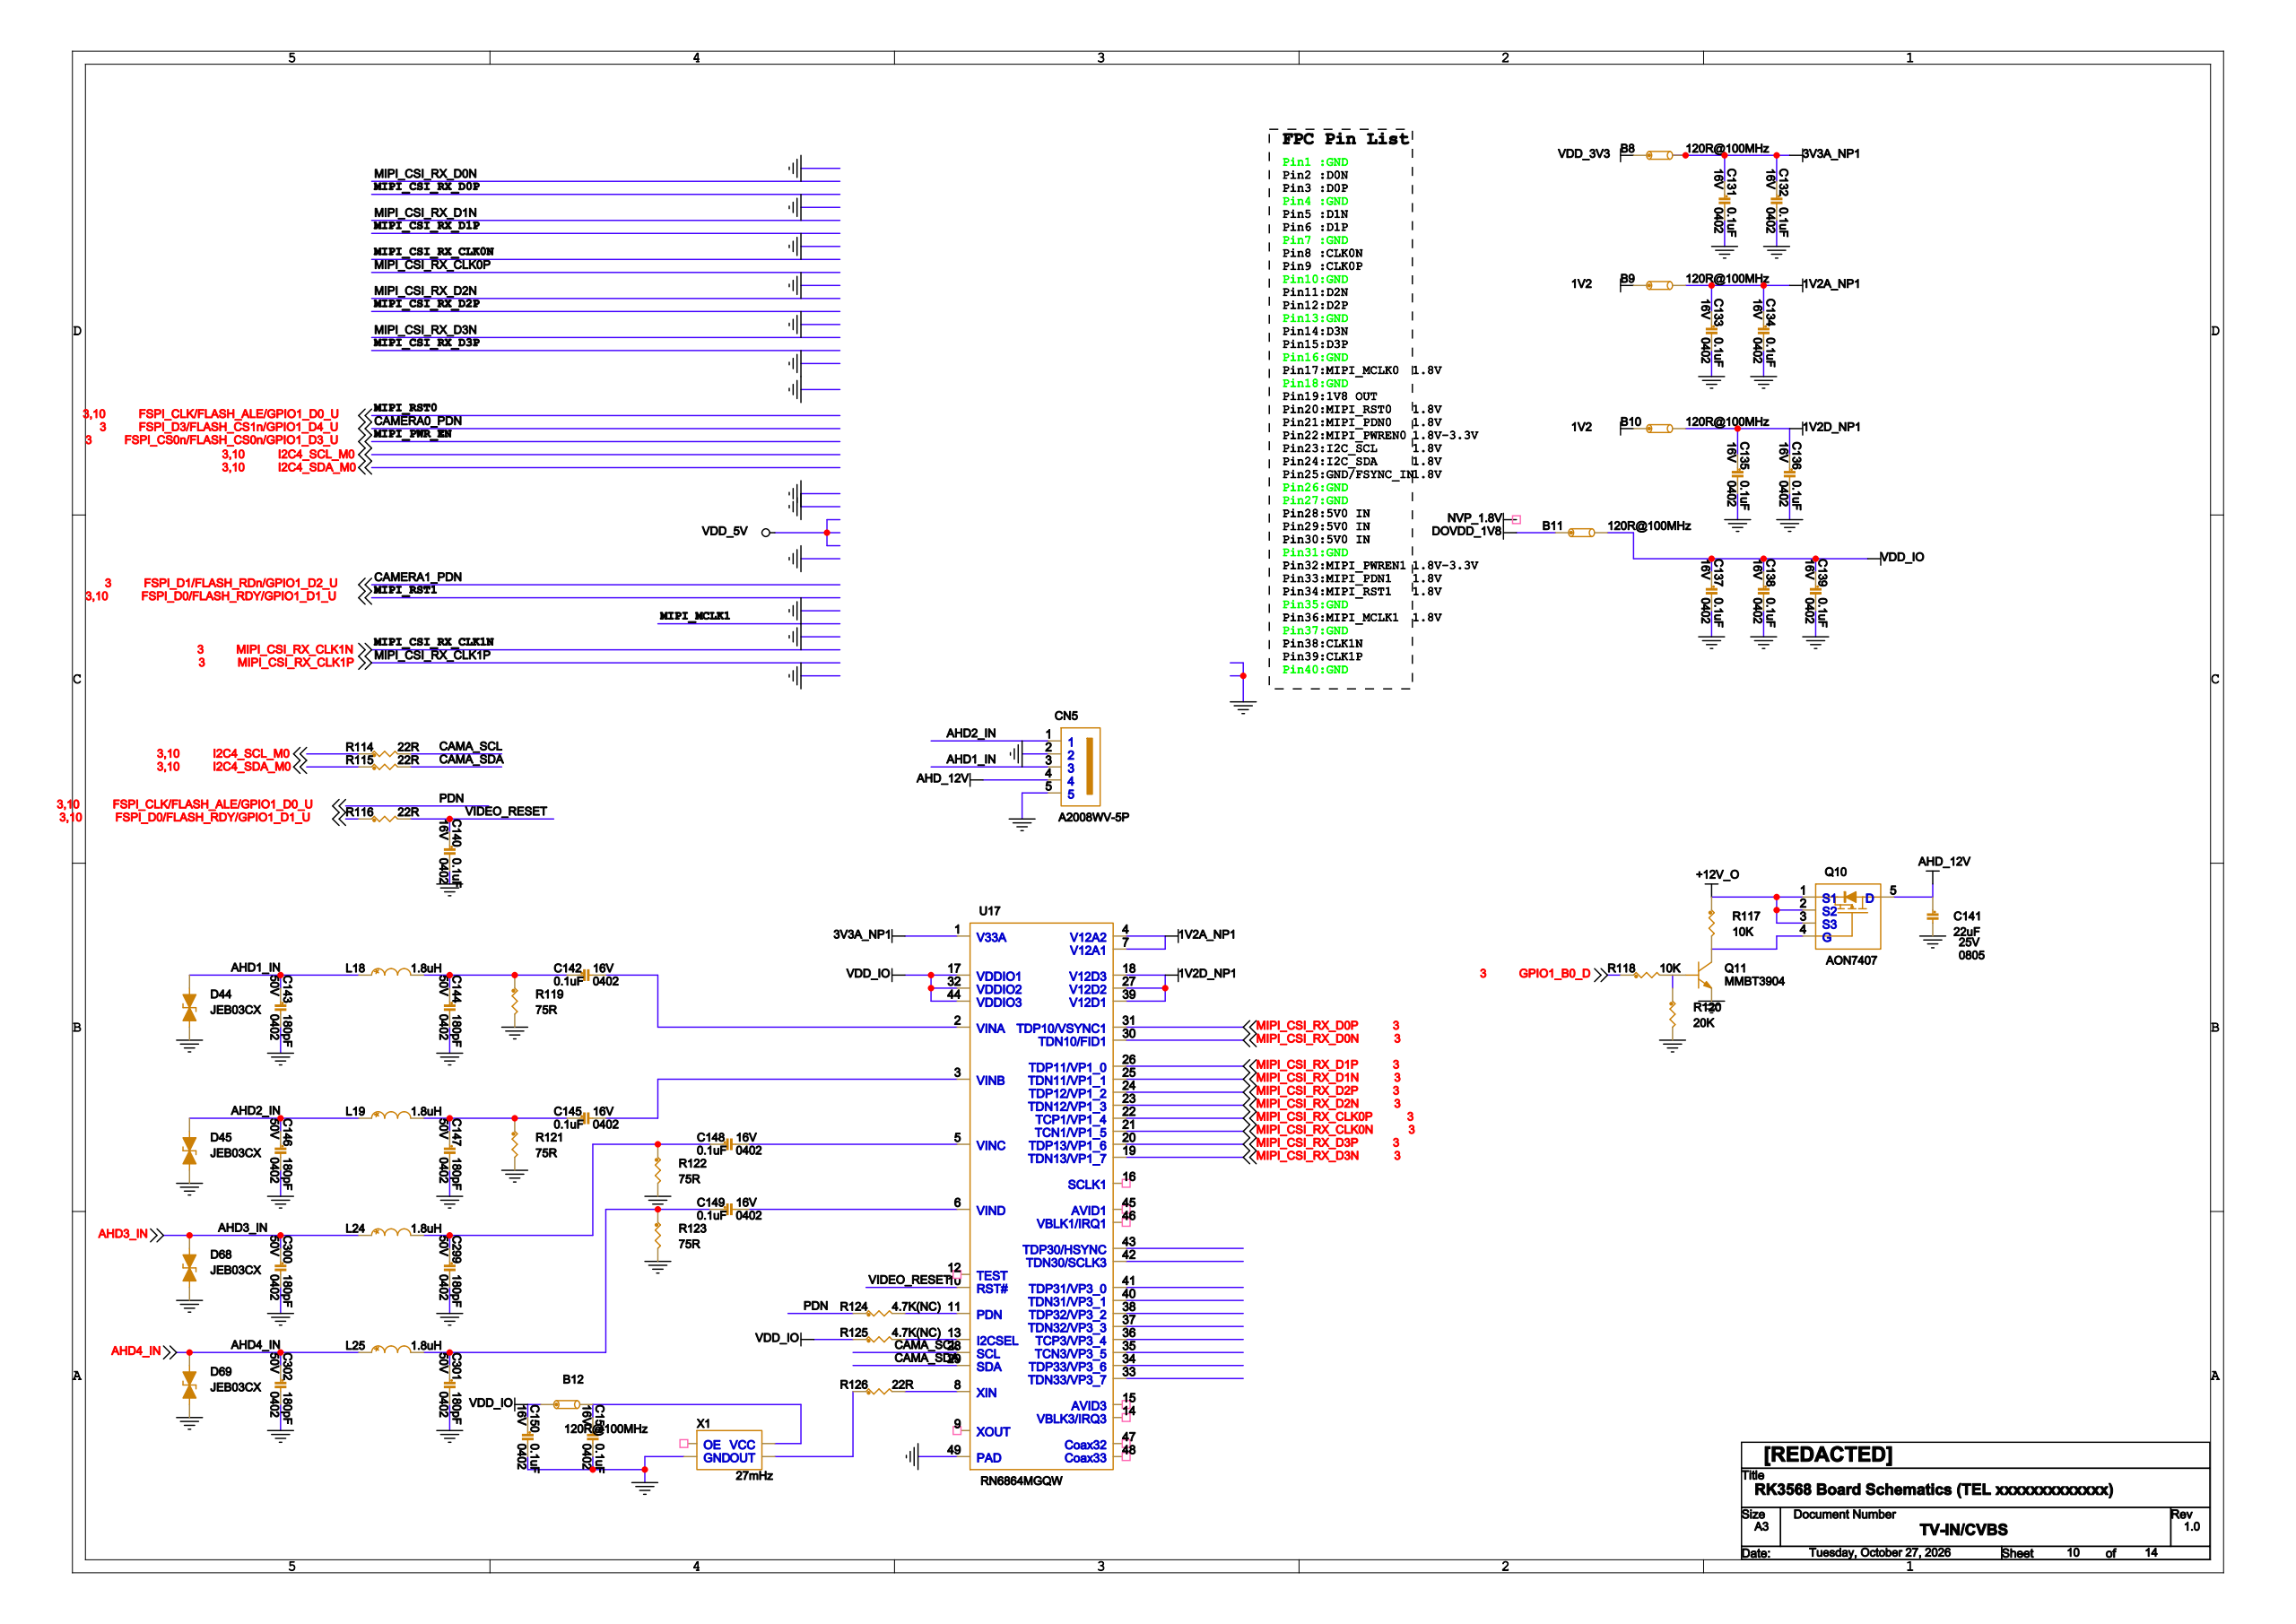Circuit board | Cadence Allegro | 669 parts | 581 nets | one sheet of the schematic
Parts on this sheet (reference | value | footprint):
B8 | 120R@100MHz | R0402
B9 | 120R@100MHz | R0402
B10 | 120R@100MHz | R0402
B11 | 120R@100MHz | R0402
B12 | 120R@100MHz | R0402
C131 | 0.1uF | C0402
C132 | 0.1uF | C0402
C133 | 0.1uF | C0402
C134 | 0.1uF | C0402
C135 | 0.1uF | C0402
C136 | 0.1uF | C0402
C137 | 0.1uF | C0402
C138 | 0.1uF | C0402
C139 | 0.1uF | C0402
C140 | 0.1uF | C0402
C141 | 22uF | C0805
C142 | 0.1uF | C0402
C143 | 180pF | C0402
C144 | 180pF | C0402
C145 | 0.1uF | C0402
C146 | 180pF | C0402
C147 | 180pF | C0402
C148 | 0.1uF | C0402
C149 | 0.1uF | C0402
C150 | 0.1uF | C0402
C151 | 0.1uF | C0402
C299 | 180pF | C0402
C300 | 180pF | C0402
C301 | 180pF | C0402
C302 | 180pF | C0402
CN5 | A2008WV-5P | A2008WV_5P
D44 | JEB03CX | SOD323
D45 | JEB03CX | SOD323
D68 | JEB03CX | SOD323
D69 | JEB03CX | SOD323
L18 | 1.8uH | R0603
L19 | 1.8uH | R0603
L24 | 1.8uH | R0603
L25 | 1.8uH | R0603
Q10 | AON7407 | DFN3X3
Q11 | MMBT3904 | SOT-23
R114 | 22R | R0402
R115 | 22R | R0402
R116 | 22R | R0402
R117 | 10K | R0402
R118 | 10K | R0402
R119 | 75R | R0402
R120 | 20K | R0402
R121 | 75R | R0402
R122 | 75R | R0402
R123 | 75R | R0402
R124 | 4.7K(NC) | R0402
R125 | 4.7K(NC) | R0402
R126 | 22R | R0402
U17 | RN6864MGQW | QFN48_0P4_6X6MM_EPAD
X1 | 27mHz | X2520
Nets of these parts (net: part-pin ...):
GND: C131-2 C132-2 C133-2 C134-2 C135-2 C136-2 C137-2 C138-2 C139-2 C140-2 C141-2 C143-2 C144-2 C146-2 C147-2 C150-2 C151-2 C299-2 C300-2 C301-2 C302-2 CN5-2 CN5-5 D44-1 D45-1 D68-1 D69-1 Q11-2 R119-2 R120-2 R121-2 R122-2 R123-2 X1-2 U17-49
VCC3V3_SYS: B8-1
+12V_O: Q10-1 Q10-2 Q10-3 R117-1
VDD_IO: B11-2 B12-1 C137-1 C138-1 C139-1 C150-1 R125-1 U17-17 U17-32 U17-44
N84266763: B12-2 C151-1 X1-4
1V2: B9-1 B10-1
1V2D_NP1: B10-2 C135-1 C136-1 U17-18 U17-27 U17-39
DOVDD_1V8: B11-1
3V3A_NP1: B8-2 C131-1 C132-1 U17-1
1V2A_NP1: B9-2 C133-1 C134-1 U17-4 U17-7
VIDEO_RESET: C140-1 R116-2 U17-10
N84266114: C142-1 C144-1 L18-2 R119-1
N84266326: C142-2 U17-2
N84608304: C145-1 C147-1 L19-2 R121-1
N84266335: C145-2 U17-3
N84266104: C148-1 C299-1 L24-2 R122-1
N84266344: C148-2 U17-5
N84266098: C149-1 C301-1 L25-2 R123-1
N84266353: C149-2 U17-6
AHD_12V: C141-1 CN5-4 Q10-5
AHD3_IN: C300-1 D68-2 L24-1
AHD4_IN: C302-1 D69-2 L25-1
AHD1_IN: C143-1 CN5-3 D44-2 L18-1
AHD2_IN: C146-1 CN5-1 D45-2 L19-1
N84360749: Q10-4 Q11-3 R117-2
I2C4_SCL_M0: R114-1
CAMA_SCL: R114-2 U17-28
I2C4_SDA_M0: R115-1
CAMA_SDA: R115-2 U17-29
FSPI_D0/FLASH_RDY/GPIO1_D1_U: R116-1
N84266745: R126-1 X1-3
N84266603: R126-2 U17-8
GPIO1_B0_D: R118-1
N84360877: Q11-1 R118-2 R120-1
FSPI_CLK/FLASH_ALE/GPIO1_D0_U: R124-1
N84266452: R124-2 U17-11
N84266498: R125-2 U17-13
MIPI_CSI_RX_CLK0N: U17-21
MIPI_CSI_RX_CLK0P: U17-22
MIPI_CSI_RX_D0N: U17-30
MIPI_CSI_RX_D1N: U17-25
MIPI_CSI_RX_D2N: U17-23
MIPI_CSI_RX_D3N: U17-19
MIPI_CSI_RX_D0P: U17-31
MIPI_CSI_RX_D1P: U17-26
MIPI_CSI_RX_D2P: U17-24
MIPI_CSI_RX_D3P: U17-20